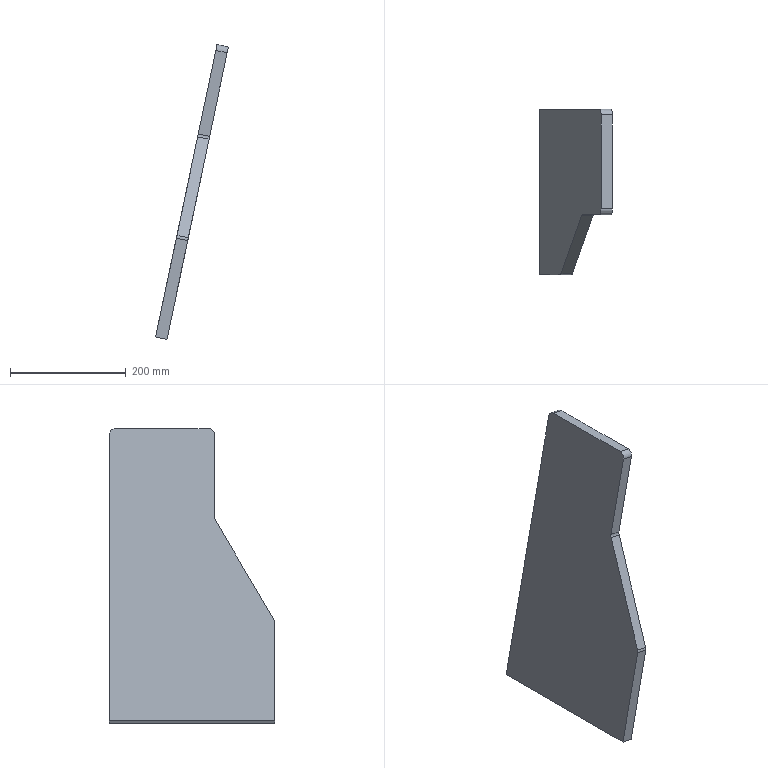Part | STEP file | 5_ESTAGIO_004-01 | 1 solid | 12 faces | box 125.479 x 285 x 508.106 mm | volume 2421288 mm3 | plane 8 | spline 4
STEP:
#1=CARTESIAN_POINT('',(0.,0.,0.));
#2=DIRECTION('',(0.,0.,1.));
#3=DIRECTION('',(1.,0.,0.));
#4=AXIS2_PLACEMENT_3D('',#1,#2,#3);
#5=CARTESIAN_POINT('',(-2789.18,-764.15,549.963));
#6=VERTEX_POINT('',#5);
#7=CARTESIAN_POINT('',(-2808.753,-764.15,554.076));
#8=VERTEX_POINT('',#7);
#9=CARTESIAN_POINT('',(-2789.18,-764.15,549.963));
#10=DIRECTION('',(-0.9786,0.,0.2056));
#11=VECTOR('',#10,1.);
#12=LINE('',#9,#11);
#13=CARTESIAN_POINT('',(-2789.18,-1049.15,549.963));
#14=DIRECTION('',(0.2056,0.,0.9786));
#15=DIRECTION('',(0.9786,0.,-0.2056));
#16=AXIS2_PLACEMENT_3D('',#13,#14,#15);
#17=PLANE('',#16);
#18=CARTESIAN_POINT('',(0.000000004,285.));
#19=DIRECTION('',(-1.,0.));
#20=VECTOR('',#19,1.);
#21=LINE('',#18,#20);
#22=(GEOMETRIC_REPRESENTATION_CONTEXT(2)PARAMETRIC_REPRESENTATION_CONTEXT()REPRESENTATION_CONTEXT('',''));
#23=DEFINITIONAL_REPRESENTATION('',(#21),#22);
#24=PCURVE('',#17,#23);
#25=CARTESIAN_POINT('',(-2789.18,-764.15,549.963));
#26=DIRECTION('',(0.,-1.,0.));
#27=DIRECTION('',(0.,0.,-1.));
#28=AXIS2_PLACEMENT_3D('',#25,#26,#27);
#29=PLANE('',#28);
#30=CARTESIAN_POINT('',(0.,0.000000004));
#31=DIRECTION('',(-0.2056,-0.9786));
#32=VECTOR('',#31,1.);
#33=LINE('',#30,#32);
#34=(GEOMETRIC_REPRESENTATION_CONTEXT(2)PARAMETRIC_REPRESENTATION_CONTEXT()REPRESENTATION_CONTEXT('',''));
#35=DEFINITIONAL_REPRESENTATION('',(#33),#34);
#36=PCURVE('',#29,#35);
#37=SURFACE_CURVE('',#12,(#24,#36),.PCURVE_S1.);
#38=EDGE_CURVE('',#6,#8,#37,.T.);
#39=ORIENTED_EDGE('',*,*,#38,.F.);
#40=CARTESIAN_POINT('',(-2789.18,-1049.15,549.963));
#41=VERTEX_POINT('',#40);
#42=CARTESIAN_POINT('',(-2789.18,-1049.15,549.963));
#43=DIRECTION('',(0.,1.,0.));
#44=VECTOR('',#43,1.);
#45=LINE('',#42,#44);
#46=CARTESIAN_POINT('',(0.,0.));
#47=DIRECTION('',(0.,1.));
#48=VECTOR('',#47,1.);
#49=LINE('',#46,#48);
#50=(GEOMETRIC_REPRESENTATION_CONTEXT(2)PARAMETRIC_REPRESENTATION_CONTEXT()REPRESENTATION_CONTEXT('',''));
#51=DEFINITIONAL_REPRESENTATION('',(#49),#50);
#52=PCURVE('',#17,#51);
#53=CARTESIAN_POINT('',(-2781.907,0.,584.575));
#54=DIRECTION('',(-0.9786,0.,0.2056));
#55=DIRECTION('',(0.2056,0.,0.9786));
#56=AXIS2_PLACEMENT_3D('',#53,#54,#55);
#57=PLANE('',#56);
#58=CARTESIAN_POINT('',(-35.367,-1049.15));
#59=DIRECTION('',(0.,1.));
#60=VECTOR('',#59,1.);
#61=LINE('',#58,#60);
#62=(GEOMETRIC_REPRESENTATION_CONTEXT(2)PARAMETRIC_REPRESENTATION_CONTEXT()REPRESENTATION_CONTEXT('',''));
#63=DEFINITIONAL_REPRESENTATION('',(#61),#62);
#64=PCURVE('',#57,#63);
#65=SURFACE_CURVE('',#45,(#52,#64),.PCURVE_S1.);
#66=EDGE_CURVE('',#41,#6,#65,.T.);
#67=ORIENTED_EDGE('',*,*,#66,.F.);
#68=CARTESIAN_POINT('',(-2808.753,-1049.15,554.076));
#69=VERTEX_POINT('',#68);
#70=CARTESIAN_POINT('',(-2789.18,-1049.15,549.963));
#71=DIRECTION('',(-0.9786,0.,0.2056));
#72=VECTOR('',#71,1.);
#73=LINE('',#70,#72);
#74=CARTESIAN_POINT('',(0.000000003,0.));
#75=DIRECTION('',(-1.,0.));
#76=VECTOR('',#75,1.);
#77=LINE('',#74,#76);
#78=(GEOMETRIC_REPRESENTATION_CONTEXT(2)PARAMETRIC_REPRESENTATION_CONTEXT()REPRESENTATION_CONTEXT('',''));
#79=DEFINITIONAL_REPRESENTATION('',(#77),#78);
#80=PCURVE('',#17,#79);
#81=CARTESIAN_POINT('',(-2753.415,-1049.15,720.165));
#82=DIRECTION('',(0.,1.,0.));
#83=DIRECTION('',(0.,0.,1.));
#84=AXIS2_PLACEMENT_3D('',#81,#82,#83);
#85=PLANE('',#84);
#86=CARTESIAN_POINT('',(-170.202,-35.765));
#87=DIRECTION('',(0.2056,-0.9786));
#88=VECTOR('',#87,1.);
#89=LINE('',#86,#88);
#90=(GEOMETRIC_REPRESENTATION_CONTEXT(2)PARAMETRIC_REPRESENTATION_CONTEXT()REPRESENTATION_CONTEXT('',''));
#91=DEFINITIONAL_REPRESENTATION('',(#89),#90);
#92=PCURVE('',#85,#91);
#93=SURFACE_CURVE('',#73,(#80,#92),.PCURVE_S1.);
#94=EDGE_CURVE('',#41,#69,#93,.T.);
#95=ORIENTED_EDGE('',*,*,#94,.T.);
#96=CARTESIAN_POINT('',(-2808.753,-1049.15,554.076));
#97=DIRECTION('',(0.,1.,0.));
#98=VECTOR('',#97,1.);
#99=LINE('',#96,#98);
#100=CARTESIAN_POINT('',(-20.,0.));
#101=DIRECTION('',(0.,1.));
#102=VECTOR('',#101,1.);
#103=LINE('',#100,#102);
#104=(GEOMETRIC_REPRESENTATION_CONTEXT(2)PARAMETRIC_REPRESENTATION_CONTEXT()REPRESENTATION_CONTEXT('',''));
#105=DEFINITIONAL_REPRESENTATION('',(#103),#104);
#106=PCURVE('',#17,#105);
#107=CARTESIAN_POINT('',(-2801.479,0.,588.687));
#108=DIRECTION('',(-0.9786,0.,0.2056));
#109=DIRECTION('',(0.2056,0.,0.9786));
#110=AXIS2_PLACEMENT_3D('',#107,#108,#109);
#111=PLANE('',#110);
#112=CARTESIAN_POINT('',(-35.367,-1049.15));
#113=DIRECTION('',(0.,1.));
#114=VECTOR('',#113,1.);
#115=LINE('',#112,#114);
#116=(GEOMETRIC_REPRESENTATION_CONTEXT(2)PARAMETRIC_REPRESENTATION_CONTEXT()REPRESENTATION_CONTEXT('',''));
#117=DEFINITIONAL_REPRESENTATION('',(#115),#116);
#118=PCURVE('',#111,#117);
#119=SURFACE_CURVE('',#99,(#106,#118),.PCURVE_S1.);
#120=EDGE_CURVE('',#69,#8,#119,.T.);
#121=ORIENTED_EDGE('',*,*,#120,.T.);
#122=EDGE_LOOP('',(#39,#67,#95,#121));
#123=FACE_BOUND('',#122,.T.);
#124=ADVANCED_FACE('',(#123),#17,.F.);
#125=ORIENTED_EDGE('',*,*,#94,.F.);
#126=CARTESIAN_POINT('',(-2753.415,-1049.15,720.165));
#127=VERTEX_POINT('',#126);
#128=CARTESIAN_POINT('',(-2753.415,-1049.15,720.165));
#129=DIRECTION('',(-0.2056,0.,-0.9786));
#130=VECTOR('',#129,1.);
#131=LINE('',#128,#130);
#132=CARTESIAN_POINT('',(-0.000000001,0.000000003));
#133=DIRECTION('',(-0.9786,-0.2056));
#134=VECTOR('',#133,1.);
#135=LINE('',#132,#134);
#136=(GEOMETRIC_REPRESENTATION_CONTEXT(2)PARAMETRIC_REPRESENTATION_CONTEXT()REPRESENTATION_CONTEXT('',''));
#137=DEFINITIONAL_REPRESENTATION('',(#135),#136);
#138=PCURVE('',#85,#137);
#139=CARTESIAN_POINT('',(138.552,-1049.15));
#140=DIRECTION('',(-1.,0.));
#141=VECTOR('',#140,1.);
#142=LINE('',#139,#141);
#143=(GEOMETRIC_REPRESENTATION_CONTEXT(2)PARAMETRIC_REPRESENTATION_CONTEXT()REPRESENTATION_CONTEXT('',''));
#144=DEFINITIONAL_REPRESENTATION('',(#142),#143);
#145=PCURVE('',#57,#144);
#146=SURFACE_CURVE('',#131,(#138,#145),.PCURVE_S1.);
#147=EDGE_CURVE('',#127,#41,#146,.T.);
#148=ORIENTED_EDGE('',*,*,#147,.F.);
#149=CARTESIAN_POINT('',(-2772.987,-1049.15,724.278));
#150=VERTEX_POINT('',#149);
#151=CARTESIAN_POINT('',(-2753.415,-1049.15,720.165));
#152=DIRECTION('',(-0.9786,0.,0.2056));
#153=VECTOR('',#152,1.);
#154=LINE('',#151,#153);
#155=CARTESIAN_POINT('',(0.,0.000000001));
#156=DIRECTION('',(0.2056,-0.9786));
#157=VECTOR('',#156,1.);
#158=LINE('',#155,#157);
#159=(GEOMETRIC_REPRESENTATION_CONTEXT(2)PARAMETRIC_REPRESENTATION_CONTEXT()REPRESENTATION_CONTEXT('',''));
#160=DEFINITIONAL_REPRESENTATION('',(#158),#159);
#161=PCURVE('',#85,#160);
#162=CARTESIAN_POINT('',(-2751.408,-1047.81,724.853));
#163=CARTESIAN_POINT('',(-2772.938,-1047.81,729.377));
#164=CARTESIAN_POINT('',(-2751.594,-1048.334,723.965));
#165=CARTESIAN_POINT('',(-2773.124,-1048.334,728.489));
#166=CARTESIAN_POINT('',(-2751.795,-1048.739,723.011));
#167=CARTESIAN_POINT('',(-2773.325,-1048.739,727.535));
#168=CARTESIAN_POINT('',(-2752.005,-1049.013,722.009));
#169=CARTESIAN_POINT('',(-2773.535,-1049.013,726.534));
#170=CARTESIAN_POINT('',(-2752.221,-1049.15,720.985));
#171=CARTESIAN_POINT('',(-2773.75,-1049.15,725.509));
#172=CARTESIAN_POINT('',(-2752.436,-1049.15,719.96));
#173=CARTESIAN_POINT('',(-2773.966,-1049.15,724.484));
#174=B_SPLINE_SURFACE_WITH_KNOTS('',5,1,((#162,#163),(#164,#165),(#166,#167),(#168,#169),(#170,#171),(#172,#173)),.UNSPECIFIED.,.F.,.F.,.F.,(6,6),(2,2),(0.,5.266),(0.,22.),.PIECEWISE_BEZIER_KNOTS.);
#175=CARTESIAN_POINT('',(5.266,1.));
#176=DIRECTION('',(0.,1.));
#177=VECTOR('',#176,1.);
#178=LINE('',#175,#177);
#179=(GEOMETRIC_REPRESENTATION_CONTEXT(2)PARAMETRIC_REPRESENTATION_CONTEXT()REPRESENTATION_CONTEXT('',''));
#180=DEFINITIONAL_REPRESENTATION('',(#178),#179);
#181=PCURVE('',#174,#180);
#182=SURFACE_CURVE('',#154,(#161,#181),.PCURVE_S1.);
#183=EDGE_CURVE('',#127,#150,#182,.T.);
#184=ORIENTED_EDGE('',*,*,#183,.T.);
#185=CARTESIAN_POINT('',(-2772.987,-1049.15,724.278));
#186=DIRECTION('',(-0.2056,0.,-0.9786));
#187=VECTOR('',#186,1.);
#188=LINE('',#185,#187);
#189=CARTESIAN_POINT('',(4.113,-19.573));
#190=DIRECTION('',(-0.9786,-0.2056));
#191=VECTOR('',#190,1.);
#192=LINE('',#189,#191);
#193=(GEOMETRIC_REPRESENTATION_CONTEXT(2)PARAMETRIC_REPRESENTATION_CONTEXT()REPRESENTATION_CONTEXT('',''));
#194=DEFINITIONAL_REPRESENTATION('',(#192),#193);
#195=PCURVE('',#85,#194);
#196=CARTESIAN_POINT('',(138.552,-1049.15));
#197=DIRECTION('',(-1.,0.));
#198=VECTOR('',#197,1.);
#199=LINE('',#196,#198);
#200=(GEOMETRIC_REPRESENTATION_CONTEXT(2)PARAMETRIC_REPRESENTATION_CONTEXT()REPRESENTATION_CONTEXT('',''));
#201=DEFINITIONAL_REPRESENTATION('',(#199),#200);
#202=PCURVE('',#111,#201);
#203=SURFACE_CURVE('',#188,(#195,#202),.PCURVE_S1.);
#204=EDGE_CURVE('',#150,#69,#203,.T.);
#205=ORIENTED_EDGE('',*,*,#204,.T.);
#206=EDGE_LOOP('',(#125,#148,#184,#205));
#207=FACE_BOUND('',#206,.T.);
#208=ADVANCED_FACE('',(#207),#85,.F.);
#209=CARTESIAN_POINT('',(-2771.959,-1047.81,729.171));
#210=VERTEX_POINT('',#209);
#211=CARTESIAN_POINT('',(-2771.959,-1047.81,729.171));
#212=CARTESIAN_POINT('',(-2772.27,-1048.683,727.692));
#213=CARTESIAN_POINT('',(-2772.628,-1049.15,725.986));
#214=CARTESIAN_POINT('',(-2772.987,-1049.15,724.278));
#215=B_SPLINE_CURVE_WITH_KNOTS('',3,(#211,#212,#213,#214),.UNSPECIFIED.,.F.,.F.,(4,4),(-0.5243,0.),.PIECEWISE_BEZIER_KNOTS.);
#216=CARTESIAN_POINT('',(0.,21.));
#217=CARTESIAN_POINT('',(5.266,21.));
#218=B_SPLINE_CURVE_WITH_KNOTS('',1,(#216,#217),.UNSPECIFIED.,.F.,.F.,(2,2),(-0.5243,0.),.PIECEWISE_BEZIER_KNOTS.);
#219=(GEOMETRIC_REPRESENTATION_CONTEXT(2)PARAMETRIC_REPRESENTATION_CONTEXT()REPRESENTATION_CONTEXT('',''));
#220=DEFINITIONAL_REPRESENTATION('',(#218),#219);
#221=PCURVE('',#174,#220);
#222=CARTESIAN_POINT('',(143.552,-1047.81));
#223=CARTESIAN_POINT('',(142.041,-1048.683));
#224=CARTESIAN_POINT('',(140.297,-1049.15));
#225=CARTESIAN_POINT('',(138.552,-1049.15));
#226=B_SPLINE_CURVE_WITH_KNOTS('',3,(#222,#223,#224,#225),.UNSPECIFIED.,.F.,.F.,(4,4),(-0.5243,0.),.PIECEWISE_BEZIER_KNOTS.);
#227=(GEOMETRIC_REPRESENTATION_CONTEXT(2)PARAMETRIC_REPRESENTATION_CONTEXT()REPRESENTATION_CONTEXT('',''));
#228=DEFINITIONAL_REPRESENTATION('',(#226),#227);
#229=PCURVE('',#111,#228);
#230=SURFACE_CURVE('',#215,(#221,#229),.PCURVE_S1.);
#231=EDGE_CURVE('',#210,#150,#230,.T.);
#232=ORIENTED_EDGE('',*,*,#231,.F.);
#233=CARTESIAN_POINT('',(-2752.386,-1047.81,725.058));
#234=VERTEX_POINT('',#233);
#235=CARTESIAN_POINT('',(-2752.386,-1047.81,725.058));
#236=DIRECTION('',(-0.9786,0.,0.2056));
#237=VECTOR('',#236,1.);
#238=LINE('',#235,#237);
#239=CARTESIAN_POINT('',(-0.000000001,1.));
#240=DIRECTION('',(0.,1.));
#241=VECTOR('',#240,1.);
#242=LINE('',#239,#241);
#243=(GEOMETRIC_REPRESENTATION_CONTEXT(2)PARAMETRIC_REPRESENTATION_CONTEXT()REPRESENTATION_CONTEXT('',''));
#244=DEFINITIONAL_REPRESENTATION('',(#242),#243);
#245=PCURVE('',#174,#244);
#246=CARTESIAN_POINT('',(-2716.654,-947.49,895.105));
#247=DIRECTION('',(-0.1028,0.866,-0.4893));
#248=DIRECTION('',(-0.9786,0.,0.2056));
#249=AXIS2_PLACEMENT_3D('',#246,#247,#248);
#250=PLANE('',#249);
#251=CARTESIAN_POINT('',(-0.000000002,-200.641));
#252=DIRECTION('',(1.,0.));
#253=VECTOR('',#252,1.);
#254=LINE('',#251,#253);
#255=(GEOMETRIC_REPRESENTATION_CONTEXT(2)PARAMETRIC_REPRESENTATION_CONTEXT()REPRESENTATION_CONTEXT('',''));
#256=DEFINITIONAL_REPRESENTATION('',(#254),#255);
#257=PCURVE('',#250,#256);
#258=SURFACE_CURVE('',#238,(#245,#257),.PCURVE_S1.);
#259=EDGE_CURVE('',#234,#210,#258,.T.);
#260=ORIENTED_EDGE('',*,*,#259,.F.);
#261=CARTESIAN_POINT('',(-2752.386,-1047.81,725.058));
#262=CARTESIAN_POINT('',(-2752.697,-1048.683,723.579));
#263=CARTESIAN_POINT('',(-2753.056,-1049.15,721.873));
#264=CARTESIAN_POINT('',(-2753.415,-1049.15,720.165));
#265=B_SPLINE_CURVE_WITH_KNOTS('',3,(#261,#262,#263,#264),.UNSPECIFIED.,.F.,.F.,(4,4),(-0.5243,0.),.PIECEWISE_BEZIER_KNOTS.);
#266=CARTESIAN_POINT('',(0.,1.));
#267=CARTESIAN_POINT('',(5.266,1.));
#268=B_SPLINE_CURVE_WITH_KNOTS('',1,(#266,#267),.UNSPECIFIED.,.F.,.F.,(2,2),(-0.5243,0.),.PIECEWISE_BEZIER_KNOTS.);
#269=(GEOMETRIC_REPRESENTATION_CONTEXT(2)PARAMETRIC_REPRESENTATION_CONTEXT()REPRESENTATION_CONTEXT('',''));
#270=DEFINITIONAL_REPRESENTATION('',(#268),#269);
#271=PCURVE('',#174,#270);
#272=CARTESIAN_POINT('',(143.552,-1047.81));
#273=CARTESIAN_POINT('',(142.041,-1048.683));
#274=CARTESIAN_POINT('',(140.297,-1049.15));
#275=CARTESIAN_POINT('',(138.552,-1049.15));
#276=B_SPLINE_CURVE_WITH_KNOTS('',3,(#272,#273,#274,#275),.UNSPECIFIED.,.F.,.F.,(4,4),(-0.5243,0.),.PIECEWISE_BEZIER_KNOTS.);
#277=(GEOMETRIC_REPRESENTATION_CONTEXT(2)PARAMETRIC_REPRESENTATION_CONTEXT()REPRESENTATION_CONTEXT('',''));
#278=DEFINITIONAL_REPRESENTATION('',(#276),#277);
#279=PCURVE('',#57,#278);
#280=SURFACE_CURVE('',#265,(#271,#279),.PCURVE_S1.);
#281=EDGE_CURVE('',#234,#127,#280,.T.);
#282=ORIENTED_EDGE('',*,*,#281,.T.);
#283=ORIENTED_EDGE('',*,*,#183,.T.);
#284=EDGE_LOOP('',(#232,#260,#282,#283));
#285=FACE_BOUND('',#284,.F.);
#286=ADVANCED_FACE('',(#285),#174,.F.);
#287=ORIENTED_EDGE('',*,*,#259,.F.);
#288=CARTESIAN_POINT('',(-2716.654,-947.49,895.105));
#289=VERTEX_POINT('',#288);
#290=CARTESIAN_POINT('',(-2716.654,-947.49,895.105));
#291=DIRECTION('',(-0.1781,-0.5,-0.8475));
#292=VECTOR('',#291,1.);
#293=LINE('',#290,#292);
#294=CARTESIAN_POINT('',(-0.000000001,0.));
#295=DIRECTION('',(0.,-1.));
#296=VECTOR('',#295,1.);
#297=LINE('',#294,#296);
#298=(GEOMETRIC_REPRESENTATION_CONTEXT(2)PARAMETRIC_REPRESENTATION_CONTEXT()REPRESENTATION_CONTEXT('',''));
#299=DEFINITIONAL_REPRESENTATION('',(#297),#298);
#300=PCURVE('',#250,#299);
#301=CARTESIAN_POINT('',(317.312,-947.49));
#302=DIRECTION('',(-0.866,-0.5));
#303=VECTOR('',#302,1.);
#304=LINE('',#301,#303);
#305=(GEOMETRIC_REPRESENTATION_CONTEXT(2)PARAMETRIC_REPRESENTATION_CONTEXT()REPRESENTATION_CONTEXT('',''));
#306=DEFINITIONAL_REPRESENTATION('',(#304),#305);
#307=PCURVE('',#57,#306);
#308=SURFACE_CURVE('',#293,(#300,#307),.PCURVE_S1.);
#309=EDGE_CURVE('',#289,#234,#308,.T.);
#310=ORIENTED_EDGE('',*,*,#309,.F.);
#311=CARTESIAN_POINT('',(-2736.226,-947.49,899.218));
#312=VERTEX_POINT('',#311);
#313=CARTESIAN_POINT('',(-2716.654,-947.49,895.105));
#314=DIRECTION('',(-0.9786,0.,0.2056));
#315=VECTOR('',#314,1.);
#316=LINE('',#313,#315);
#317=CARTESIAN_POINT('',(-0.000000002,0.000000001));
#318=DIRECTION('',(1.,0.));
#319=VECTOR('',#318,1.);
#320=LINE('',#317,#319);
#321=(GEOMETRIC_REPRESENTATION_CONTEXT(2)PARAMETRIC_REPRESENTATION_CONTEXT()REPRESENTATION_CONTEXT('',''));
#322=DEFINITIONAL_REPRESENTATION('',(#320),#321);
#323=PCURVE('',#250,#322);
#324=CARTESIAN_POINT('',(-2714.647,-946.15,899.792));
#325=CARTESIAN_POINT('',(-2736.177,-946.15,904.317));
#326=CARTESIAN_POINT('',(-2714.862,-946.15,898.768));
#327=CARTESIAN_POINT('',(-2736.392,-946.15,903.292));
#328=CARTESIAN_POINT('',(-2715.078,-946.287,897.743));
#329=CARTESIAN_POINT('',(-2736.608,-946.287,902.267));
#330=CARTESIAN_POINT('',(-2715.288,-946.561,896.742));
#331=CARTESIAN_POINT('',(-2736.818,-946.561,901.266));
#332=CARTESIAN_POINT('',(-2715.489,-946.966,895.787));
#333=CARTESIAN_POINT('',(-2737.018,-946.966,900.311));
#334=CARTESIAN_POINT('',(-2715.675,-947.49,894.899));
#335=CARTESIAN_POINT('',(-2737.205,-947.49,899.423));
#336=B_SPLINE_SURFACE_WITH_KNOTS('',5,1,((#324,#325),(#326,#327),(#328,#329),(#330,#331),(#332,#333),(#334,#335)),.UNSPECIFIED.,.F.,.F.,.F.,(6,6),(2,2),(0.,5.266),(0.,22.),.PIECEWISE_BEZIER_KNOTS.);
#337=CARTESIAN_POINT('',(5.266,1.));
#338=DIRECTION('',(0.,1.));
#339=VECTOR('',#338,1.);
#340=LINE('',#337,#339);
#341=(GEOMETRIC_REPRESENTATION_CONTEXT(2)PARAMETRIC_REPRESENTATION_CONTEXT()REPRESENTATION_CONTEXT('',''));
#342=DEFINITIONAL_REPRESENTATION('',(#340),#341);
#343=PCURVE('',#336,#342);
#344=SURFACE_CURVE('',#316,(#323,#343),.PCURVE_S1.);
#345=EDGE_CURVE('',#289,#312,#344,.T.);
#346=ORIENTED_EDGE('',*,*,#345,.T.);
#347=CARTESIAN_POINT('',(-2736.226,-947.49,899.218));
#348=DIRECTION('',(-0.1781,-0.5,-0.8475));
#349=VECTOR('',#348,1.);
#350=LINE('',#347,#349);
#351=CARTESIAN_POINT('',(20.,0.000000001));
#352=DIRECTION('',(0.,-1.));
#353=VECTOR('',#352,1.);
#354=LINE('',#351,#353);
#355=(GEOMETRIC_REPRESENTATION_CONTEXT(2)PARAMETRIC_REPRESENTATION_CONTEXT()REPRESENTATION_CONTEXT('',''));
#356=DEFINITIONAL_REPRESENTATION('',(#354),#355);
#357=PCURVE('',#250,#356);
#358=CARTESIAN_POINT('',(317.312,-947.49));
#359=DIRECTION('',(-0.866,-0.5));
#360=VECTOR('',#359,1.);
#361=LINE('',#358,#360);
#362=(GEOMETRIC_REPRESENTATION_CONTEXT(2)PARAMETRIC_REPRESENTATION_CONTEXT()REPRESENTATION_CONTEXT('',''));
#363=DEFINITIONAL_REPRESENTATION('',(#361),#362);
#364=PCURVE('',#111,#363);
#365=SURFACE_CURVE('',#350,(#357,#364),.PCURVE_S1.);
#366=EDGE_CURVE('',#312,#210,#365,.T.);
#367=ORIENTED_EDGE('',*,*,#366,.T.);
#368=EDGE_LOOP('',(#287,#310,#346,#367));
#369=FACE_BOUND('',#368,.T.);
#370=ADVANCED_FACE('',(#369),#250,.F.);
#371=CARTESIAN_POINT('',(-2735.198,-946.15,904.111));
#372=VERTEX_POINT('',#371);
#373=CARTESIAN_POINT('',(-2735.198,-946.15,904.111));
#374=CARTESIAN_POINT('',(-2735.557,-946.15,902.403));
#375=CARTESIAN_POINT('',(-2735.916,-946.617,900.697));
#376=CARTESIAN_POINT('',(-2736.226,-947.49,899.218));
#377=B_SPLINE_CURVE_WITH_KNOTS('',3,(#373,#374,#375,#376),.UNSPECIFIED.,.F.,.F.,(4,4),(-0.5243,0.),.PIECEWISE_BEZIER_KNOTS.);
#378=CARTESIAN_POINT('',(0.,21.));
#379=CARTESIAN_POINT('',(5.266,21.));
#380=B_SPLINE_CURVE_WITH_KNOTS('',1,(#378,#379),.UNSPECIFIED.,.F.,.F.,(2,2),(-0.5243,0.),.PIECEWISE_BEZIER_KNOTS.);
#381=(GEOMETRIC_REPRESENTATION_CONTEXT(2)PARAMETRIC_REPRESENTATION_CONTEXT()REPRESENTATION_CONTEXT('',''));
#382=DEFINITIONAL_REPRESENTATION('',(#380),#381);
#383=PCURVE('',#336,#382);
#384=CARTESIAN_POINT('',(322.312,-946.15));
#385=CARTESIAN_POINT('',(320.567,-946.15));
#386=CARTESIAN_POINT('',(318.824,-946.617));
#387=CARTESIAN_POINT('',(317.312,-947.49));
#388=B_SPLINE_CURVE_WITH_KNOTS('',3,(#384,#385,#386,#387),.UNSPECIFIED.,.F.,.F.,(4,4),(-0.5243,0.),.PIECEWISE_BEZIER_KNOTS.);
#389=(GEOMETRIC_REPRESENTATION_CONTEXT(2)PARAMETRIC_REPRESENTATION_CONTEXT()REPRESENTATION_CONTEXT('',''));
#390=DEFINITIONAL_REPRESENTATION('',(#388),#389);
#391=PCURVE('',#111,#390);
#392=SURFACE_CURVE('',#377,(#383,#391),.PCURVE_S1.);
#393=EDGE_CURVE('',#372,#312,#392,.T.);
#394=ORIENTED_EDGE('',*,*,#393,.F.);
#395=CARTESIAN_POINT('',(-2715.626,-946.15,899.998));
#396=VERTEX_POINT('',#395);
#397=CARTESIAN_POINT('',(-2715.626,-946.15,899.998));
#398=DIRECTION('',(-0.9786,0.,0.2056));
#399=VECTOR('',#398,1.);
#400=LINE('',#397,#399);
#401=CARTESIAN_POINT('',(-0.000000001,1.));
#402=DIRECTION('',(0.,1.));
#403=VECTOR('',#402,1.);
#404=LINE('',#401,#403);
#405=(GEOMETRIC_REPRESENTATION_CONTEXT(2)PARAMETRIC_REPRESENTATION_CONTEXT()REPRESENTATION_CONTEXT('',''));
#406=DEFINITIONAL_REPRESENTATION('',(#404),#405);
#407=PCURVE('',#336,#406);
#408=CARTESIAN_POINT('',(-2685.33,-946.15,1044.17));
#409=DIRECTION('',(0.,1.,0.));
#410=DIRECTION('',(0.,0.,1.));
#411=AXIS2_PLACEMENT_3D('',#408,#409,#410);
#412=PLANE('',#411);
#413=CARTESIAN_POINT('',(-144.172,-30.295));
#414=DIRECTION('',(0.2056,-0.9786));
#415=VECTOR('',#414,1.);
#416=LINE('',#413,#415);
#417=(GEOMETRIC_REPRESENTATION_CONTEXT(2)PARAMETRIC_REPRESENTATION_CONTEXT()REPRESENTATION_CONTEXT('',''));
#418=DEFINITIONAL_REPRESENTATION('',(#416),#417);
#419=PCURVE('',#412,#418);
#420=SURFACE_CURVE('',#400,(#407,#419),.PCURVE_S1.);
#421=EDGE_CURVE('',#396,#372,#420,.T.);
#422=ORIENTED_EDGE('',*,*,#421,.F.);
#423=CARTESIAN_POINT('',(-2715.626,-946.15,899.998));
#424=CARTESIAN_POINT('',(-2715.985,-946.15,898.29));
#425=CARTESIAN_POINT('',(-2716.343,-946.617,896.584));
#426=CARTESIAN_POINT('',(-2716.654,-947.49,895.105));
#427=B_SPLINE_CURVE_WITH_KNOTS('',3,(#423,#424,#425,#426),.UNSPECIFIED.,.F.,.F.,(4,4),(-0.5243,0.),.PIECEWISE_BEZIER_KNOTS.);
#428=CARTESIAN_POINT('',(0.,1.));
#429=CARTESIAN_POINT('',(5.266,1.));
#430=B_SPLINE_CURVE_WITH_KNOTS('',1,(#428,#429),.UNSPECIFIED.,.F.,.F.,(2,2),(-0.5243,0.),.PIECEWISE_BEZIER_KNOTS.);
#431=(GEOMETRIC_REPRESENTATION_CONTEXT(2)PARAMETRIC_REPRESENTATION_CONTEXT()REPRESENTATION_CONTEXT('',''));
#432=DEFINITIONAL_REPRESENTATION('',(#430),#431);
#433=PCURVE('',#336,#432);
#434=CARTESIAN_POINT('',(322.312,-946.15));
#435=CARTESIAN_POINT('',(320.567,-946.15));
#436=CARTESIAN_POINT('',(318.824,-946.617));
#437=CARTESIAN_POINT('',(317.312,-947.49));
#438=B_SPLINE_CURVE_WITH_KNOTS('',3,(#434,#435,#436,#437),.UNSPECIFIED.,.F.,.F.,(4,4),(-0.5243,0.),.PIECEWISE_BEZIER_KNOTS.);
#439=(GEOMETRIC_REPRESENTATION_CONTEXT(2)PARAMETRIC_REPRESENTATION_CONTEXT()REPRESENTATION_CONTEXT('',''));
#440=DEFINITIONAL_REPRESENTATION('',(#438),#439);
#441=PCURVE('',#57,#440);
#442=SURFACE_CURVE('',#427,(#433,#441),.PCURVE_S1.);
#443=EDGE_CURVE('',#396,#289,#442,.T.);
#444=ORIENTED_EDGE('',*,*,#443,.T.);
#445=ORIENTED_EDGE('',*,*,#345,.T.);
#446=EDGE_LOOP('',(#394,#422,#444,#445));
#447=FACE_BOUND('',#446,.F.);
#448=ADVANCED_FACE('',(#447),#336,.F.);
#449=ORIENTED_EDGE('',*,*,#421,.F.);
#450=CARTESIAN_POINT('',(-2685.33,-946.15,1044.17));
#451=VERTEX_POINT('',#450);
#452=CARTESIAN_POINT('',(-2685.33,-946.15,1044.17));
#453=DIRECTION('',(-0.2056,0.,-0.9786));
#454=VECTOR('',#453,1.);
#455=LINE('',#452,#454);
#456=CARTESIAN_POINT('',(0.,-0.000000002));
#457=DIRECTION('',(-0.9786,-0.2056));
#458=VECTOR('',#457,1.);
#459=LINE('',#456,#458);
#460=(GEOMETRIC_REPRESENTATION_CONTEXT(2)PARAMETRIC_REPRESENTATION_CONTEXT()REPRESENTATION_CONTEXT('',''));
#461=DEFINITIONAL_REPRESENTATION('',(#459),#460);
#462=PCURVE('',#412,#461);
#463=CARTESIAN_POINT('',(469.633,-946.15));
#464=DIRECTION('',(-1.,0.));
#465=VECTOR('',#464,1.);
#466=LINE('',#463,#465);
#467=(GEOMETRIC_REPRESENTATION_CONTEXT(2)PARAMETRIC_REPRESENTATION_CONTEXT()REPRESENTATION_CONTEXT('',''));
#468=DEFINITIONAL_REPRESENTATION('',(#466),#467);
#469=PCURVE('',#57,#468);
#470=SURFACE_CURVE('',#455,(#462,#469),.PCURVE_S1.);
#471=EDGE_CURVE('',#451,#396,#470,.T.);
#472=ORIENTED_EDGE('',*,*,#471,.F.);
#473=CARTESIAN_POINT('',(-2704.903,-946.15,1048.283));
#474=VERTEX_POINT('',#473);
#475=CARTESIAN_POINT('',(-2685.33,-946.15,1044.17));
#476=DIRECTION('',(-0.9786,0.,0.2056));
#477=VECTOR('',#476,1.);
#478=LINE('',#475,#477);
#479=CARTESIAN_POINT('',(0.,-0.000000001));
#480=DIRECTION('',(0.2056,-0.9786));
#481=VECTOR('',#480,1.);
#482=LINE('',#479,#481);
#483=(GEOMETRIC_REPRESENTATION_CONTEXT(2)PARAMETRIC_REPRESENTATION_CONTEXT()REPRESENTATION_CONTEXT('',''));
#484=DEFINITIONAL_REPRESENTATION('',(#482),#483);
#485=PCURVE('',#412,#484);
#486=CARTESIAN_POINT('',(-2682.295,-936.15,1053.75));
#487=CARTESIAN_POINT('',(-2703.825,-936.15,1058.275));
#488=CARTESIAN_POINT('',(-2682.295,-939.292,1053.75));
#489=CARTESIAN_POINT('',(-2703.825,-939.292,1058.275));
#490=CARTESIAN_POINT('',(-2682.548,-942.436,1052.547));
#491=CARTESIAN_POINT('',(-2704.078,-942.436,1057.071));
#492=CARTESIAN_POINT('',(-2683.059,-944.92,1050.116));
#493=CARTESIAN_POINT('',(-2704.589,-944.92,1054.64));
#494=CARTESIAN_POINT('',(-2683.705,-946.15,1047.039));
#495=CARTESIAN_POINT('',(-2705.235,-946.15,1051.563));
#496=CARTESIAN_POINT('',(-2684.352,-946.15,1043.964));
#497=CARTESIAN_POINT('',(-2705.881,-946.15,1048.488));
#498=B_SPLINE_SURFACE_WITH_KNOTS('',5,1,((#486,#487),(#488,#489),(#490,#491),(#492,#493),(#494,#495),(#496,#497)),.UNSPECIFIED.,.F.,.F.,.F.,(6,6),(2,2),(0.,16.549),(0.,22.),.PIECEWISE_BEZIER_KNOTS.);
#499=CARTESIAN_POINT('',(16.549,1.));
#500=DIRECTION('',(0.,1.));
#501=VECTOR('',#500,1.);
#502=LINE('',#499,#501);
#503=(GEOMETRIC_REPRESENTATION_CONTEXT(2)PARAMETRIC_REPRESENTATION_CONTEXT()REPRESENTATION_CONTEXT('',''));
#504=DEFINITIONAL_REPRESENTATION('',(#502),#503);
#505=PCURVE('',#498,#504);
#506=SURFACE_CURVE('',#478,(#485,#505),.PCURVE_S1.);
#507=EDGE_CURVE('',#451,#474,#506,.T.);
#508=ORIENTED_EDGE('',*,*,#507,.T.);
#509=CARTESIAN_POINT('',(-2704.903,-946.15,1048.283));
#510=DIRECTION('',(-0.2056,0.,-0.9786));
#511=VECTOR('',#510,1.);
#512=LINE('',#509,#511);
#513=CARTESIAN_POINT('',(4.113,-19.573));
#514=DIRECTION('',(-0.9786,-0.2056));
#515=VECTOR('',#514,1.);
#516=LINE('',#513,#515);
#517=(GEOMETRIC_REPRESENTATION_CONTEXT(2)PARAMETRIC_REPRESENTATION_CONTEXT()REPRESENTATION_CONTEXT('',''));
#518=DEFINITIONAL_REPRESENTATION('',(#516),#517);
#519=PCURVE('',#412,#518);
#520=CARTESIAN_POINT('',(469.633,-946.15));
#521=DIRECTION('',(-1.,0.));
#522=VECTOR('',#521,1.);
#523=LINE('',#520,#522);
#524=(GEOMETRIC_REPRESENTATION_CONTEXT(2)PARAMETRIC_REPRESENTATION_CONTEXT()REPRESENTATION_CONTEXT('',''));
#525=DEFINITIONAL_REPRESENTATION('',(#523),#524);
#526=PCURVE('',#111,#525);
#527=SURFACE_CURVE('',#512,(#519,#526),.PCURVE_S1.);
#528=EDGE_CURVE('',#474,#372,#527,.T.);
#529=ORIENTED_EDGE('',*,*,#528,.T.);
#530=EDGE_LOOP('',(#449,#472,#508,#529));
#531=FACE_BOUND('',#530,.T.);
#532=ADVANCED_FACE('',(#531),#412,.F.);
#533=CARTESIAN_POINT('',(-2702.846,-936.15,1058.069));
#534=VERTEX_POINT('',#533);
#535=CARTESIAN_POINT('',(-2702.846,-936.15,1058.069));
#536=CARTESIAN_POINT('',(-2702.846,-938.624,1058.069));
#537=CARTESIAN_POINT('',(-2703.043,-941.086,1057.131));
#538=CARTESIAN_POINT('',(-2703.387,-942.909,1055.494));
#539=CARTESIAN_POINT('',(-2703.732,-944.736,1053.855));
#540=CARTESIAN_POINT('',(-2704.22,-945.904,1051.53));
#541=CARTESIAN_POINT('',(-2704.728,-946.114,1049.113));
#542=CARTESIAN_POINT('',(-2704.786,-946.138,1048.837));
#543=CARTESIAN_POINT('',(-2704.844,-946.15,1048.56));
#544=CARTESIAN_POINT('',(-2704.903,-946.15,1048.283));
#545=B_SPLINE_CURVE_WITH_KNOTS('',3,(#535,#536,#537,#538,#539,#540,#541,#542,#543,#544),.UNSPECIFIED.,.F.,.F.,(4,3,3,4),(682.708,690.131,697.567,698.416),.UNSPECIFIED.);
#546=CARTESIAN_POINT('',(0.,21.));
#547=CARTESIAN_POINT('',(16.549,21.));
#548=B_SPLINE_CURVE_WITH_KNOTS('',1,(#546,#547),.UNSPECIFIED.,.F.,.F.,(2,2),(682.708,698.416),.PIECEWISE_BEZIER_KNOTS.);
#549=(GEOMETRIC_REPRESENTATION_CONTEXT(2)PARAMETRIC_REPRESENTATION_CONTEXT()REPRESENTATION_CONTEXT('',''));
#550=DEFINITIONAL_REPRESENTATION('',(#548),#549);
#551=PCURVE('',#498,#550);
#552=CARTESIAN_POINT('',(479.633,-936.15));
#553=CARTESIAN_POINT('',(479.633,-938.624));
#554=CARTESIAN_POINT('',(478.674,-941.086));
#555=CARTESIAN_POINT('',(477.002,-942.909));
#556=CARTESIAN_POINT('',(475.326,-944.736));
#557=CARTESIAN_POINT('',(472.951,-945.904));
#558=CARTESIAN_POINT('',(470.481,-946.114));
#559=CARTESIAN_POINT('',(470.199,-946.138));
#560=CARTESIAN_POINT('',(469.916,-946.15));
#561=CARTESIAN_POINT('',(469.633,-946.15));
#562=B_SPLINE_CURVE_WITH_KNOTS('',3,(#552,#553,#554,#555,#556,#557,#558,#559,#560,#561),.UNSPECIFIED.,.F.,.F.,(4,3,3,4),(682.708,690.131,697.567,698.416),.UNSPECIFIED.);
#563=(GEOMETRIC_REPRESENTATION_CONTEXT(2)PARAMETRIC_REPRESENTATION_CONTEXT()REPRESENTATION_CONTEXT('',''));
#564=DEFINITIONAL_REPRESENTATION('',(#562),#563);
#565=PCURVE('',#111,#564);
#566=SURFACE_CURVE('',#545,(#551,#565),.PCURVE_S1.);
#567=EDGE_CURVE('',#534,#474,#566,.T.);
#568=ORIENTED_EDGE('',*,*,#567,.F.);
#569=CARTESIAN_POINT('',(-2683.274,-936.15,1053.956));
#570=VERTEX_POINT('',#569);
#571=CARTESIAN_POINT('',(-2683.274,-936.15,1053.956));
#572=DIRECTION('',(-0.9786,0.,0.2056));
#573=VECTOR('',#572,1.);
#574=LINE('',#571,#573);
#575=CARTESIAN_POINT('',(0.,1.));
#576=DIRECTION('',(0.,1.));
#577=VECTOR('',#576,1.);
#578=LINE('',#575,#577);
#579=(GEOMETRIC_REPRESENTATION_CONTEXT(2)PARAMETRIC_REPRESENTATION_CONTEXT()REPRESENTATION_CONTEXT('',''));
#580=DEFINITIONAL_REPRESENTATION('',(#578),#579);
#581=PCURVE('',#498,#580);
#582=CARTESIAN_POINT('',(-2683.274,-774.15,1053.956));
#583=DIRECTION('',(-0.2056,0.,-0.9786));
#584=DIRECTION('',(-0.9786,0.,0.2056));
#585=AXIS2_PLACEMENT_3D('',#582,#583,#584);
#586=PLANE('',#585);
#587=CARTESIAN_POINT('',(0.,-162.));
#588=DIRECTION('',(1.,0.));
#589=VECTOR('',#588,1.);
#590=LINE('',#587,#589);
#591=(GEOMETRIC_REPRESENTATION_CONTEXT(2)PARAMETRIC_REPRESENTATION_CONTEXT()REPRESENTATION_CONTEXT('',''));
#592=DEFINITIONAL_REPRESENTATION('',(#590),#591);
#593=PCURVE('',#586,#592);
#594=SURFACE_CURVE('',#574,(#581,#593),.PCURVE_S1.);
#595=EDGE_CURVE('',#570,#534,#594,.T.);
#596=ORIENTED_EDGE('',*,*,#595,.F.);
#597=CARTESIAN_POINT('',(-2683.274,-936.15,1053.956));
#598=CARTESIAN_POINT('',(-2683.274,-939.292,1053.956));
#599=CARTESIAN_POINT('',(-2683.527,-942.436,1052.752));
#600=CARTESIAN_POINT('',(-2684.037,-944.92,1050.322));
#601=CARTESIAN_POINT('',(-2684.684,-946.15,1047.244));
#602=CARTESIAN_POINT('',(-2685.33,-946.15,1044.17));
#603=B_SPLINE_CURVE_WITH_KNOTS('',5,(#597,#598,#599,#600,#601,#602),.UNSPECIFIED.,.F.,.F.,(6,6),(682.708,698.416),.PIECEWISE_BEZIER_KNOTS.);
#604=CARTESIAN_POINT('',(0.,1.));
#605=CARTESIAN_POINT('',(16.549,1.));
#606=B_SPLINE_CURVE_WITH_KNOTS('',1,(#604,#605),.UNSPECIFIED.,.F.,.F.,(2,2),(682.708,698.416),.PIECEWISE_BEZIER_KNOTS.);
#607=(GEOMETRIC_REPRESENTATION_CONTEXT(2)PARAMETRIC_REPRESENTATION_CONTEXT()REPRESENTATION_CONTEXT('',''));
#608=DEFINITIONAL_REPRESENTATION('',(#606),#607);
#609=PCURVE('',#498,#608);
#610=CARTESIAN_POINT('',(479.633,-936.15));
#611=CARTESIAN_POINT('',(479.633,-939.292));
#612=CARTESIAN_POINT('',(478.403,-942.436));
#613=CARTESIAN_POINT('',(475.919,-944.92));
#614=CARTESIAN_POINT('',(472.774,-946.15));
#615=CARTESIAN_POINT('',(469.633,-946.15));
#616=B_SPLINE_CURVE_WITH_KNOTS('',5,(#610,#611,#612,#613,#614,#615),.UNSPECIFIED.,.F.,.F.,(6,6),(682.708,698.416),.PIECEWISE_BEZIER_KNOTS.);
#617=(GEOMETRIC_REPRESENTATION_CONTEXT(2)PARAMETRIC_REPRESENTATION_CONTEXT()REPRESENTATION_CONTEXT('',''));
#618=DEFINITIONAL_REPRESENTATION('',(#616),#617);
#619=PCURVE('',#57,#618);
#620=SURFACE_CURVE('',#603,(#609,#619),.PCURVE_S1.);
#621=EDGE_CURVE('',#570,#451,#620,.T.);
#622=ORIENTED_EDGE('',*,*,#621,.T.);
#623=ORIENTED_EDGE('',*,*,#507,.T.);
#624=EDGE_LOOP('',(#568,#596,#622,#623));
#625=FACE_BOUND('',#624,.F.);
#626=ADVANCED_FACE('',(#625),#498,.F.);
#627=ORIENTED_EDGE('',*,*,#595,.F.);
#628=CARTESIAN_POINT('',(-2683.274,-774.15,1053.956));
#629=VERTEX_POINT('',#628);
#630=CARTESIAN_POINT('',(-2683.274,-774.15,1053.956));
#631=DIRECTION('',(0.,-1.,0.));
#632=VECTOR('',#631,1.);
#633=LINE('',#630,#632);
#634=CARTESIAN_POINT('',(0.,0.));
#635=DIRECTION('',(0.,-1.));
#636=VECTOR('',#635,1.);
#637=LINE('',#634,#636);
#638=(GEOMETRIC_REPRESENTATION_CONTEXT(2)PARAMETRIC_REPRESENTATION_CONTEXT()REPRESENTATION_CONTEXT('',''));
#639=DEFINITIONAL_REPRESENTATION('',(#637),#638);
#640=PCURVE('',#586,#639);
#641=CARTESIAN_POINT('',(479.633,-774.15));
#642=DIRECTION('',(0.,-1.));
#643=VECTOR('',#642,1.);
#644=LINE('',#641,#643);
#645=(GEOMETRIC_REPRESENTATION_CONTEXT(2)PARAMETRIC_REPRESENTATION_CONTEXT()REPRESENTATION_CONTEXT('',''));
#646=DEFINITIONAL_REPRESENTATION('',(#644),#645);
#647=PCURVE('',#57,#646);
#648=SURFACE_CURVE('',#633,(#640,#647),.PCURVE_S1.);
#649=EDGE_CURVE('',#629,#570,#648,.T.);
#650=ORIENTED_EDGE('',*,*,#649,.F.);
#651=CARTESIAN_POINT('',(-2702.846,-774.15,1058.069));
#652=VERTEX_POINT('',#651);
#653=CARTESIAN_POINT('',(-2683.274,-774.15,1053.956));
#654=DIRECTION('',(-0.9786,0.,0.2056));
#655=VECTOR('',#654,1.);
#656=LINE('',#653,#655);
#657=CARTESIAN_POINT('',(0.,0.));
#658=DIRECTION('',(1.,0.));
#659=VECTOR('',#658,1.);
#660=LINE('',#657,#659);
#661=(GEOMETRIC_REPRESENTATION_CONTEXT(2)PARAMETRIC_REPRESENTATION_CONTEXT()REPRESENTATION_CONTEXT('',''));
#662=DEFINITIONAL_REPRESENTATION('',(#660),#661);
#663=PCURVE('',#586,#662);
#664=CARTESIAN_POINT('',(-2684.352,-764.15,1043.964));
#665=CARTESIAN_POINT('',(-2705.881,-764.15,1048.488));
#666=CARTESIAN_POINT('',(-2683.705,-764.15,1047.039));
#667=CARTESIAN_POINT('',(-2705.235,-764.15,1051.563));
#668=CARTESIAN_POINT('',(-2683.059,-765.38,1050.116));
#669=CARTESIAN_POINT('',(-2704.589,-765.38,1054.64));
#670=CARTESIAN_POINT('',(-2682.548,-767.864,1052.547));
#671=CARTESIAN_POINT('',(-2704.078,-767.864,1057.071));
#672=CARTESIAN_POINT('',(-2682.295,-771.008,1053.75));
#673=CARTESIAN_POINT('',(-2703.825,-771.008,1058.275));
#674=CARTESIAN_POINT('',(-2682.295,-774.15,1053.75));
#675=CARTESIAN_POINT('',(-2703.825,-774.15,1058.275));
#676=B_SPLINE_SURFACE_WITH_KNOTS('',5,1,((#664,#665),(#666,#667),(#668,#669),(#670,#671),(#672,#673),(#674,#675)),.UNSPECIFIED.,.F.,.F.,.F.,(6,6),(2,2),(0.,16.549),(0.,22.),.PIECEWISE_BEZIER_KNOTS.);
#677=CARTESIAN_POINT('',(16.549,1.));
#678=DIRECTION('',(0.,1.));
#679=VECTOR('',#678,1.);
#680=LINE('',#677,#679);
#681=(GEOMETRIC_REPRESENTATION_CONTEXT(2)PARAMETRIC_REPRESENTATION_CONTEXT()REPRESENTATION_CONTEXT('',''));
#682=DEFINITIONAL_REPRESENTATION('',(#680),#681);
#683=PCURVE('',#676,#682);
#684=SURFACE_CURVE('',#656,(#663,#683),.PCURVE_S1.);
#685=EDGE_CURVE('',#629,#652,#684,.T.);
#686=ORIENTED_EDGE('',*,*,#685,.T.);
#687=CARTESIAN_POINT('',(-2702.846,-774.15,1058.069));
#688=DIRECTION('',(0.,-1.,0.));
#689=VECTOR('',#688,1.);
#690=LINE('',#687,#689);
#691=CARTESIAN_POINT('',(20.,0.));
#692=DIRECTION('',(0.,-1.));
#693=VECTOR('',#692,1.);
#694=LINE('',#691,#693);
#695=(GEOMETRIC_REPRESENTATION_CONTEXT(2)PARAMETRIC_REPRESENTATION_CONTEXT()REPRESENTATION_CONTEXT('',''));
#696=DEFINITIONAL_REPRESENTATION('',(#694),#695);
#697=PCURVE('',#586,#696);
#698=CARTESIAN_POINT('',(479.633,-774.15));
#699=DIRECTION('',(0.,-1.));
#700=VECTOR('',#699,1.);
#701=LINE('',#698,#700);
#702=(GEOMETRIC_REPRESENTATION_CONTEXT(2)PARAMETRIC_REPRESENTATION_CONTEXT()REPRESENTATION_CONTEXT('',''));
#703=DEFINITIONAL_REPRESENTATION('',(#701),#702);
#704=PCURVE('',#111,#703);
#705=SURFACE_CURVE('',#690,(#697,#704),.PCURVE_S1.);
#706=EDGE_CURVE('',#652,#534,#705,.T.);
#707=ORIENTED_EDGE('',*,*,#706,.T.);
#708=EDGE_LOOP('',(#627,#650,#686,#707));
#709=FACE_BOUND('',#708,.T.);
#710=ADVANCED_FACE('',(#709),#586,.F.);
#711=CARTESIAN_POINT('',(-2704.903,-764.15,1048.283));
#712=VERTEX_POINT('',#711);
#713=CARTESIAN_POINT('',(-2704.903,-764.15,1048.283));
#714=CARTESIAN_POINT('',(-2704.394,-764.15,1050.704));
#715=CARTESIAN_POINT('',(-2703.888,-765.108,1053.113));
#716=CARTESIAN_POINT('',(-2703.513,-766.781,1054.898));
#717=CARTESIAN_POINT('',(-2703.137,-768.456,1056.685));
#718=CARTESIAN_POINT('',(-2702.897,-770.832,1057.828));
#719=CARTESIAN_POINT('',(-2702.854,-773.302,1058.034));
#720=CARTESIAN_POINT('',(-2702.849,-773.584,1058.057));
#721=CARTESIAN_POINT('',(-2702.846,-773.867,1058.069));
#722=CARTESIAN_POINT('',(-2702.846,-774.15,1058.069));
#723=B_SPLINE_CURVE_WITH_KNOTS('',3,(#713,#714,#715,#716,#717,#718,#719,#720,#721,#722),.UNSPECIFIED.,.F.,.F.,(4,3,3,4),(505.,512.423,519.859,520.708),.UNSPECIFIED.);
#724=CARTESIAN_POINT('',(0.000000002,21.));
#725=CARTESIAN_POINT('',(16.549,21.));
#726=B_SPLINE_CURVE_WITH_KNOTS('',1,(#724,#725),.UNSPECIFIED.,.F.,.F.,(2,2),(505.,520.708),.PIECEWISE_BEZIER_KNOTS.);
#727=(GEOMETRIC_REPRESENTATION_CONTEXT(2)PARAMETRIC_REPRESENTATION_CONTEXT()REPRESENTATION_CONTEXT('',''));
#728=DEFINITIONAL_REPRESENTATION('',(#726),#727);
#729=PCURVE('',#676,#728);
#730=CARTESIAN_POINT('',(469.633,-764.15));
#731=CARTESIAN_POINT('',(472.107,-764.15));
#732=CARTESIAN_POINT('',(474.569,-765.108));
#733=CARTESIAN_POINT('',(476.392,-766.781));
#734=CARTESIAN_POINT('',(478.219,-768.456));
#735=CARTESIAN_POINT('',(479.387,-770.832));
#736=CARTESIAN_POINT('',(479.597,-773.302));
#737=CARTESIAN_POINT('',(479.621,-773.584));
#738=CARTESIAN_POINT('',(479.633,-773.867));
#739=CARTESIAN_POINT('',(479.633,-774.15));
#740=B_SPLINE_CURVE_WITH_KNOTS('',3,(#730,#731,#732,#733,#734,#735,#736,#737,#738,#739),.UNSPECIFIED.,.F.,.F.,(4,3,3,4),(505.,512.423,519.859,520.708),.UNSPECIFIED.);
#741=(GEOMETRIC_REPRESENTATION_CONTEXT(2)PARAMETRIC_REPRESENTATION_CONTEXT()REPRESENTATION_CONTEXT('',''));
#742=DEFINITIONAL_REPRESENTATION('',(#740),#741);
#743=PCURVE('',#111,#742);
#744=SURFACE_CURVE('',#723,(#729,#743),.PCURVE_S1.);
#745=EDGE_CURVE('',#712,#652,#744,.T.);
#746=ORIENTED_EDGE('',*,*,#745,.F.);
#747=CARTESIAN_POINT('',(-2685.33,-764.15,1044.17));
#748=VERTEX_POINT('',#747);
#749=CARTESIAN_POINT('',(-2685.33,-764.15,1044.17));
#750=DIRECTION('',(-0.9786,0.,0.2056));
#751=VECTOR('',#750,1.);
#752=LINE('',#749,#751);
#753=CARTESIAN_POINT('',(0.,1.));
#754=DIRECTION('',(0.,1.));
#755=VECTOR('',#754,1.);
#756=LINE('',#753,#755);
#757=(GEOMETRIC_REPRESENTATION_CONTEXT(2)PARAMETRIC_REPRESENTATION_CONTEXT()REPRESENTATION_CONTEXT('',''));
#758=DEFINITIONAL_REPRESENTATION('',(#756),#757);
#759=PCURVE('',#676,#758);
#760=CARTESIAN_POINT('',(-494.207,103.85));
#761=DIRECTION('',(-0.2056,-0.9786));
#762=VECTOR('',#761,1.);
#763=LINE('',#760,#762);
#764=(GEOMETRIC_REPRESENTATION_CONTEXT(2)PARAMETRIC_REPRESENTATION_CONTEXT()REPRESENTATION_CONTEXT('',''));
#765=DEFINITIONAL_REPRESENTATION('',(#763),#764);
#766=PCURVE('',#29,#765);
#767=SURFACE_CURVE('',#752,(#759,#766),.PCURVE_S1.);
#768=EDGE_CURVE('',#748,#712,#767,.T.);
#769=ORIENTED_EDGE('',*,*,#768,.F.);
#770=CARTESIAN_POINT('',(-2685.33,-764.15,1044.17));
#771=CARTESIAN_POINT('',(-2684.684,-764.15,1047.244));
#772=CARTESIAN_POINT('',(-2684.037,-765.38,1050.322));
#773=CARTESIAN_POINT('',(-2683.527,-767.864,1052.752));
#774=CARTESIAN_POINT('',(-2683.274,-771.008,1053.956));
#775=CARTESIAN_POINT('',(-2683.274,-774.15,1053.956));
#776=B_SPLINE_CURVE_WITH_KNOTS('',5,(#770,#771,#772,#773,#774,#775),.UNSPECIFIED.,.F.,.F.,(6,6),(505.,520.708),.PIECEWISE_BEZIER_KNOTS.);
#777=CARTESIAN_POINT('',(0.,1.));
#778=CARTESIAN_POINT('',(16.549,1.));
#779=B_SPLINE_CURVE_WITH_KNOTS('',1,(#777,#778),.UNSPECIFIED.,.F.,.F.,(2,2),(505.,520.708),.PIECEWISE_BEZIER_KNOTS.);
#780=(GEOMETRIC_REPRESENTATION_CONTEXT(2)PARAMETRIC_REPRESENTATION_CONTEXT()REPRESENTATION_CONTEXT('',''));
#781=DEFINITIONAL_REPRESENTATION('',(#779),#780);
#782=PCURVE('',#676,#781);
#783=CARTESIAN_POINT('',(469.633,-764.15));
#784=CARTESIAN_POINT('',(472.774,-764.15));
#785=CARTESIAN_POINT('',(475.919,-765.38));
#786=CARTESIAN_POINT('',(478.403,-767.864));
#787=CARTESIAN_POINT('',(479.633,-771.008));
#788=CARTESIAN_POINT('',(479.633,-774.15));
#789=B_SPLINE_CURVE_WITH_KNOTS('',5,(#783,#784,#785,#786,#787,#788),.UNSPECIFIED.,.F.,.F.,(6,6),(505.,520.708),.PIECEWISE_BEZIER_KNOTS.);
#790=(GEOMETRIC_REPRESENTATION_CONTEXT(2)PARAMETRIC_REPRESENTATION_CONTEXT()REPRESENTATION_CONTEXT('',''));
#791=DEFINITIONAL_REPRESENTATION('',(#789),#790);
#792=PCURVE('',#57,#791);
#793=SURFACE_CURVE('',#776,(#782,#792),.PCURVE_S1.);
#794=EDGE_CURVE('',#748,#629,#793,.T.);
#795=ORIENTED_EDGE('',*,*,#794,.T.);
#796=ORIENTED_EDGE('',*,*,#685,.T.);
#797=EDGE_LOOP('',(#746,#769,#795,#796));
#798=FACE_BOUND('',#797,.F.);
#799=ADVANCED_FACE('',(#798),#676,.F.);
#800=ORIENTED_EDGE('',*,*,#768,.F.);
#801=CARTESIAN_POINT('',(-2789.18,-764.15,549.963));
#802=DIRECTION('',(0.2056,0.,0.9786));
#803=VECTOR('',#802,1.);
#804=LINE('',#801,#803);
#805=CARTESIAN_POINT('',(0.000000001,0.000000008));
#806=DIRECTION('',(-0.9786,0.2056));
#807=VECTOR('',#806,1.);
#808=LINE('',#805,#807);
#809=(GEOMETRIC_REPRESENTATION_CONTEXT(2)PARAMETRIC_REPRESENTATION_CONTEXT()REPRESENTATION_CONTEXT('',''));
#810=DEFINITIONAL_REPRESENTATION('',(#808),#809);
#811=PCURVE('',#29,#810);
#812=CARTESIAN_POINT('',(-35.367,-764.15));
#813=DIRECTION('',(1.,0.));
#814=VECTOR('',#813,1.);
#815=LINE('',#812,#814);
#816=(GEOMETRIC_REPRESENTATION_CONTEXT(2)PARAMETRIC_REPRESENTATION_CONTEXT()REPRESENTATION_CONTEXT('',''));
#817=DEFINITIONAL_REPRESENTATION('',(#815),#816);
#818=PCURVE('',#57,#817);
#819=SURFACE_CURVE('',#804,(#811,#818),.PCURVE_S1.);
#820=EDGE_CURVE('',#6,#748,#819,.T.);
#821=ORIENTED_EDGE('',*,*,#820,.F.);
#822=ORIENTED_EDGE('',*,*,#38,.T.);
#823=CARTESIAN_POINT('',(-2808.753,-764.15,554.076));
#824=DIRECTION('',(0.2056,0.,0.9786));
#825=VECTOR('',#824,1.);
#826=LINE('',#823,#825);
#827=CARTESIAN_POINT('',(-4.113,-19.573));
#828=DIRECTION('',(-0.9786,0.2056));
#829=VECTOR('',#828,1.);
#830=LINE('',#827,#829);
#831=(GEOMETRIC_REPRESENTATION_CONTEXT(2)PARAMETRIC_REPRESENTATION_CONTEXT()REPRESENTATION_CONTEXT('',''));
#832=DEFINITIONAL_REPRESENTATION('',(#830),#831);
#833=PCURVE('',#29,#832);
#834=CARTESIAN_POINT('',(-35.367,-764.15));
#835=DIRECTION('',(1.,0.));
#836=VECTOR('',#835,1.);
#837=LINE('',#834,#836);
#838=(GEOMETRIC_REPRESENTATION_CONTEXT(2)PARAMETRIC_REPRESENTATION_CONTEXT()REPRESENTATION_CONTEXT('',''));
#839=DEFINITIONAL_REPRESENTATION('',(#837),#838);
#840=PCURVE('',#111,#839);
#841=SURFACE_CURVE('',#826,(#833,#840),.PCURVE_S1.);
#842=EDGE_CURVE('',#8,#712,#841,.T.);
#843=ORIENTED_EDGE('',*,*,#842,.T.);
#844=EDGE_LOOP('',(#800,#821,#822,#843));
#845=FACE_BOUND('',#844,.T.);
#846=ADVANCED_FACE('',(#845),#29,.F.);
#847=ORIENTED_EDGE('',*,*,#820,.T.);
#848=ORIENTED_EDGE('',*,*,#794,.T.);
#849=ORIENTED_EDGE('',*,*,#649,.T.);
#850=ORIENTED_EDGE('',*,*,#621,.T.);
#851=ORIENTED_EDGE('',*,*,#471,.T.);
#852=ORIENTED_EDGE('',*,*,#443,.T.);
#853=ORIENTED_EDGE('',*,*,#309,.T.);
#854=ORIENTED_EDGE('',*,*,#281,.T.);
#855=ORIENTED_EDGE('',*,*,#147,.T.);
#856=ORIENTED_EDGE('',*,*,#66,.T.);
#857=EDGE_LOOP('',(#847,#848,#849,#850,#851,#852,#853,#854,#855,#856));
#858=FACE_BOUND('',#857,.T.);
#859=ADVANCED_FACE('',(#858),#57,.F.);
#860=ORIENTED_EDGE('',*,*,#120,.F.);
#861=ORIENTED_EDGE('',*,*,#204,.F.);
#862=ORIENTED_EDGE('',*,*,#231,.F.);
#863=ORIENTED_EDGE('',*,*,#366,.F.);
#864=ORIENTED_EDGE('',*,*,#393,.F.);
#865=ORIENTED_EDGE('',*,*,#528,.F.);
#866=ORIENTED_EDGE('',*,*,#567,.F.);
#867=ORIENTED_EDGE('',*,*,#706,.F.);
#868=ORIENTED_EDGE('',*,*,#745,.F.);
#869=ORIENTED_EDGE('',*,*,#842,.F.);
#870=EDGE_LOOP('',(#860,#861,#862,#863,#864,#865,#866,#867,#868,#869));
#871=FACE_BOUND('',#870,.T.);
#872=ADVANCED_FACE('',(#871),#111,.T.);
#873=CLOSED_SHELL('',(#124,#208,#286,#370,#448,#532,#626,#710,#799,#846,#859,#872));
#874=MANIFOLD_SOLID_BREP('',#873);
#875=(LENGTH_UNIT()NAMED_UNIT(*)SI_UNIT(.MILLI.,.METRE.));
#876=UNCERTAINTY_MEASURE_WITH_UNIT(LENGTH_MEASURE(0.002),#875,'','');
#877=(NAMED_UNIT(*)PLANE_ANGLE_UNIT()SI_UNIT($,.RADIAN.));
#878=(NAMED_UNIT(*)SI_UNIT($,.STERADIAN.)SOLID_ANGLE_UNIT());
#879=(GEOMETRIC_REPRESENTATION_CONTEXT(3)GLOBAL_UNCERTAINTY_ASSIGNED_CONTEXT((#876))GLOBAL_UNIT_ASSIGNED_CONTEXT((#875,#877,#878))REPRESENTATION_CONTEXT('',''));
#880=ADVANCED_BREP_SHAPE_REPRESENTATION('',(#4,#874),#879);